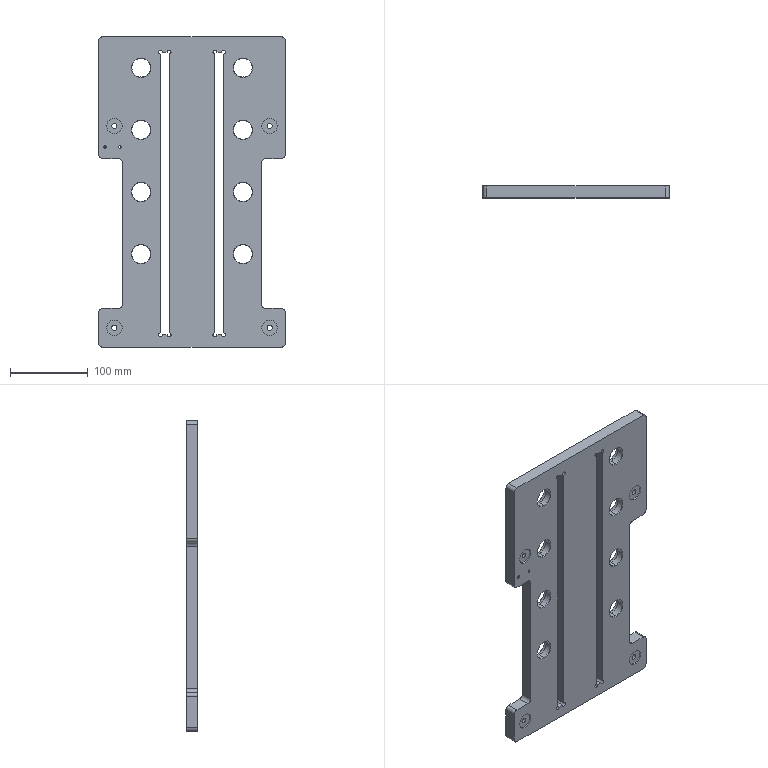Part | STEP file | PN_0018 | 1 solid | 170 faces | box 240 x 15 x 400 mm | volume 1068440 mm3 | cylinder 84 | cone 48 | plane 38 | commonest cylinder face diameters 24.05 x16 31.1 x16 5 x12 10 x12 6.6 x8 11 x8